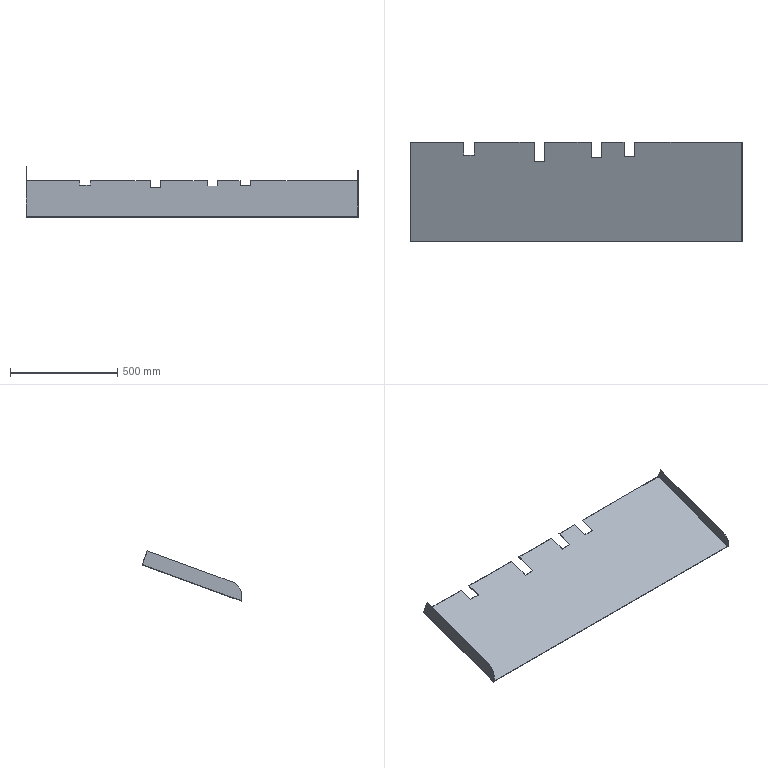Part | NX | features solid 2 | 1 solid | 28 faces | box 1550 x 466.287 x 233.957 mm | volume 1602943 mm3 | plane 26 | cylinder 2 | commonest cylinder face diameters 100 x1 140 x1
STEP:
#1=CARTESIAN_POINT('',(-650.,-738.618,-498.246));
#2=VERTEX_POINT('',#1);
#3=CARTESIAN_POINT('',(-370.,-738.618,-498.246));
#4=VERTEX_POINT('',#3);
#5=CARTESIAN_POINT('',(108.81,-738.618,-498.246));
#6=DIRECTION('',(-1.,0.,0.));
#7=VECTOR('',#6,1000.);
#8=LINE('',#5,#7);
#9=EDGE_CURVE('',#2,#4,#8,.F.);
#10=ORIENTED_EDGE('',*,*,#9,.T.);
#11=CARTESIAN_POINT('',(-370.,-737.934,-500.125));
#12=VERTEX_POINT('',#11);
#13=CARTESIAN_POINT('',(-370.,-738.618,-498.246));
#14=DIRECTION('',(0.,-0.342,0.9397));
#15=VECTOR('',#14,1000.);
#16=LINE('',#13,#15);
#17=EDGE_CURVE('',#4,#12,#16,.F.);
#18=ORIENTED_EDGE('',*,*,#17,.T.);
#19=CARTESIAN_POINT('',(-650.,-737.934,-500.125));
#20=VERTEX_POINT('',#19);
#21=CARTESIAN_POINT('',(108.81,-737.934,-500.125));
#22=DIRECTION('',(-1.,0.,0.));
#23=VECTOR('',#22,1000.);
#24=LINE('',#21,#23);
#25=EDGE_CURVE('',#20,#12,#24,.F.);
#26=ORIENTED_EDGE('',*,*,#25,.F.);
#27=CARTESIAN_POINT('',(-650.,-738.618,-498.246));
#28=DIRECTION('',(0.,-0.342,0.9397));
#29=VECTOR('',#28,1000.);
#30=LINE('',#27,#29);
#31=EDGE_CURVE('',#20,#2,#30,.T.);
#32=ORIENTED_EDGE('',*,*,#31,.T.);
#33=EDGE_LOOP('',(#10,#18,#26,#32));
#34=FACE_BOUND('',#33,.T.);
#35=CARTESIAN_POINT('',(108.81,-738.618,-498.246));
#36=DIRECTION('',(0.,0.9397,0.342));
#37=DIRECTION('',(1.,0.,0.));
#38=AXIS2_PLACEMENT_3D('',#35,#36,#37);
#39=PLANE('',#38);
#40=ADVANCED_FACE('',(#34),#39,.T.);
#41=CARTESIAN_POINT('',(-55.,-737.934,-500.125));
#42=VERTEX_POINT('',#41);
#43=CARTESIAN_POINT('',(49.,-737.934,-500.125));
#44=VERTEX_POINT('',#43);
#45=CARTESIAN_POINT('',(108.81,-737.934,-500.125));
#46=DIRECTION('',(-1.,0.,0.));
#47=VECTOR('',#46,1000.);
#48=LINE('',#45,#47);
#49=EDGE_CURVE('',#42,#44,#48,.F.);
#50=ORIENTED_EDGE('',*,*,#49,.F.);
#51=CARTESIAN_POINT('',(-55.,-738.618,-498.246));
#52=VERTEX_POINT('',#51);
#53=CARTESIAN_POINT('',(-55.,-738.618,-498.246));
#54=DIRECTION('',(0.,-0.342,0.9397));
#55=VECTOR('',#54,1000.);
#56=LINE('',#53,#55);
#57=EDGE_CURVE('',#42,#52,#56,.T.);
#58=ORIENTED_EDGE('',*,*,#57,.T.);
#59=CARTESIAN_POINT('',(49.,-738.618,-498.246));
#60=VERTEX_POINT('',#59);
#61=CARTESIAN_POINT('',(108.81,-738.618,-498.246));
#62=DIRECTION('',(-1.,0.,0.));
#63=VECTOR('',#62,1000.);
#64=LINE('',#61,#63);
#65=EDGE_CURVE('',#52,#60,#64,.F.);
#66=ORIENTED_EDGE('',*,*,#65,.T.);
#67=CARTESIAN_POINT('',(49.,-738.618,-498.246));
#68=DIRECTION('',(0.,0.342,-0.9397));
#69=VECTOR('',#68,1000.);
#70=LINE('',#67,#69);
#71=EDGE_CURVE('',#60,#44,#70,.T.);
#72=ORIENTED_EDGE('',*,*,#71,.T.);
#73=EDGE_LOOP('',(#50,#58,#66,#72));
#74=FACE_BOUND('',#73,.T.);
#75=CARTESIAN_POINT('',(108.81,-738.618,-498.246));
#76=DIRECTION('',(0.,0.9397,0.342));
#77=DIRECTION('',(1.,0.,0.));
#78=AXIS2_PLACEMENT_3D('',#75,#76,#77);
#79=PLANE('',#78);
#80=ADVANCED_FACE('',(#74),#79,.T.);
#81=CARTESIAN_POINT('',(-320.,-737.934,-500.125));
#82=VERTEX_POINT('',#81);
#83=CARTESIAN_POINT('',(-105.,-737.934,-500.125));
#84=VERTEX_POINT('',#83);
#85=CARTESIAN_POINT('',(108.81,-737.934,-500.125));
#86=DIRECTION('',(-1.,0.,0.));
#87=VECTOR('',#86,1000.);
#88=LINE('',#85,#87);
#89=EDGE_CURVE('',#82,#84,#88,.F.);
#90=ORIENTED_EDGE('',*,*,#89,.F.);
#91=CARTESIAN_POINT('',(-320.,-738.618,-498.246));
#92=VERTEX_POINT('',#91);
#93=CARTESIAN_POINT('',(-320.,-738.618,-498.246));
#94=DIRECTION('',(0.,-0.342,0.9397));
#95=VECTOR('',#94,1000.);
#96=LINE('',#93,#95);
#97=EDGE_CURVE('',#82,#92,#96,.T.);
#98=ORIENTED_EDGE('',*,*,#97,.T.);
#99=CARTESIAN_POINT('',(-105.,-738.618,-498.246));
#100=VERTEX_POINT('',#99);
#101=CARTESIAN_POINT('',(108.81,-738.618,-498.246));
#102=DIRECTION('',(-1.,0.,0.));
#103=VECTOR('',#102,1000.);
#104=LINE('',#101,#103);
#105=EDGE_CURVE('',#92,#100,#104,.F.);
#106=ORIENTED_EDGE('',*,*,#105,.T.);
#107=CARTESIAN_POINT('',(-105.,-738.618,-498.246));
#108=DIRECTION('',(0.,-0.342,0.9397));
#109=VECTOR('',#108,1000.);
#110=LINE('',#107,#109);
#111=EDGE_CURVE('',#100,#84,#110,.F.);
#112=ORIENTED_EDGE('',*,*,#111,.T.);
#113=EDGE_LOOP('',(#90,#98,#106,#112));
#114=FACE_BOUND('',#113,.T.);
#115=CARTESIAN_POINT('',(108.81,-738.618,-498.246));
#116=DIRECTION('',(0.,0.9397,0.342));
#117=DIRECTION('',(1.,0.,0.));
#118=AXIS2_PLACEMENT_3D('',#115,#116,#117);
#119=PLANE('',#118);
#120=ADVANCED_FACE('',(#114),#119,.T.);
#121=CARTESIAN_POINT('',(-948.,-738.618,-498.246));
#122=VERTEX_POINT('',#121);
#123=CARTESIAN_POINT('',(-700.,-738.618,-498.246));
#124=VERTEX_POINT('',#123);
#125=CARTESIAN_POINT('',(108.81,-738.618,-498.246));
#126=DIRECTION('',(-1.,0.,0.));
#127=VECTOR('',#126,1000.);
#128=LINE('',#125,#127);
#129=EDGE_CURVE('',#122,#124,#128,.F.);
#130=ORIENTED_EDGE('',*,*,#129,.T.);
#131=CARTESIAN_POINT('',(-700.,-737.934,-500.125));
#132=VERTEX_POINT('',#131);
#133=CARTESIAN_POINT('',(-700.,-738.618,-498.246));
#134=DIRECTION('',(0.,-0.342,0.9397));
#135=VECTOR('',#134,1000.);
#136=LINE('',#133,#135);
#137=EDGE_CURVE('',#124,#132,#136,.F.);
#138=ORIENTED_EDGE('',*,*,#137,.T.);
#139=CARTESIAN_POINT('',(-950.,-737.934,-500.125));
#140=VERTEX_POINT('',#139);
#141=CARTESIAN_POINT('',(108.81,-737.934,-500.125));
#142=DIRECTION('',(-1.,0.,0.));
#143=VECTOR('',#142,1000.);
#144=LINE('',#141,#143);
#145=EDGE_CURVE('',#140,#132,#144,.F.);
#146=ORIENTED_EDGE('',*,*,#145,.F.);
#147=CARTESIAN_POINT('',(-950.,-761.876,-434.347));
#148=VERTEX_POINT('',#147);
#149=CARTESIAN_POINT('',(-950.,-745.859,-478.352));
#150=DIRECTION('',(0.,-0.342,0.9397));
#151=VECTOR('',#150,1000.);
#152=LINE('',#149,#151);
#153=EDGE_CURVE('',#148,#140,#152,.F.);
#154=ORIENTED_EDGE('',*,*,#153,.F.);
#155=CARTESIAN_POINT('',(-948.,-761.876,-434.347));
#156=VERTEX_POINT('',#155);
#157=CARTESIAN_POINT('',(-950.,-761.876,-434.347));
#158=DIRECTION('',(1.,0.,0.));
#159=VECTOR('',#158,1000.);
#160=LINE('',#157,#159);
#161=EDGE_CURVE('',#148,#156,#160,.T.);
#162=ORIENTED_EDGE('',*,*,#161,.T.);
#163=CARTESIAN_POINT('',(-948.,-737.934,-500.125));
#164=DIRECTION('',(0.,0.342,-0.9397));
#165=VECTOR('',#164,1000.);
#166=LINE('',#163,#165);
#167=EDGE_CURVE('',#122,#156,#166,.F.);
#168=ORIENTED_EDGE('',*,*,#167,.F.);
#169=EDGE_LOOP('',(#130,#138,#146,#154,#162,#168));
#170=FACE_BOUND('',#169,.T.);
#171=CARTESIAN_POINT('',(108.81,-738.618,-498.246));
#172=DIRECTION('',(0.,0.9397,0.342));
#173=DIRECTION('',(1.,0.,0.));
#174=AXIS2_PLACEMENT_3D('',#171,#172,#173);
#175=PLANE('',#174);
#176=ADVANCED_FACE('',(#170),#175,.T.);
#177=CARTESIAN_POINT('',(-948.,-1200.,-668.304));
#178=VERTEX_POINT('',#177);
#179=CARTESIAN_POINT('',(597.803,-1200.,-668.304));
#180=VERTEX_POINT('',#179);
#181=CARTESIAN_POINT('',(108.81,-1200.,-668.304));
#182=DIRECTION('',(1.,0.,0.));
#183=VECTOR('',#182,1000.);
#184=LINE('',#181,#183);
#185=EDGE_CURVE('',#178,#180,#184,.T.);
#186=ORIENTED_EDGE('',*,*,#185,.T.);
#187=CARTESIAN_POINT('',(597.803,-1200.,-666.175));
#188=VERTEX_POINT('',#187);
#189=CARTESIAN_POINT('',(597.803,-1200.,-700.));
#190=DIRECTION('',(0.,0.,1.));
#191=VECTOR('',#190,1000.);
#192=LINE('',#189,#191);
#193=EDGE_CURVE('',#180,#188,#192,.T.);
#194=ORIENTED_EDGE('',*,*,#193,.T.);
#195=CARTESIAN_POINT('',(-948.,-1200.,-666.175));
#196=VERTEX_POINT('',#195);
#197=CARTESIAN_POINT('',(108.81,-1200.,-666.175));
#198=DIRECTION('',(1.,0.,0.));
#199=VECTOR('',#198,1000.);
#200=LINE('',#197,#199);
#201=EDGE_CURVE('',#196,#188,#200,.T.);
#202=ORIENTED_EDGE('',*,*,#201,.F.);
#203=CARTESIAN_POINT('',(-948.,-1200.,-700.));
#204=DIRECTION('',(0.,0.,1.));
#205=VECTOR('',#204,1000.);
#206=LINE('',#203,#205);
#207=EDGE_CURVE('',#178,#196,#206,.T.);
#208=ORIENTED_EDGE('',*,*,#207,.F.);
#209=EDGE_LOOP('',(#186,#194,#202,#208));
#210=FACE_BOUND('',#209,.T.);
#211=CARTESIAN_POINT('',(-1915.,-1200.,-700.));
#212=DIRECTION('',(0.,1.,0.));
#213=DIRECTION('',(-1.,0.,0.));
#214=AXIS2_PLACEMENT_3D('',#211,#212,#213);
#215=PLANE('',#214);
#216=ADVANCED_FACE('',(#210),#215,.F.);
#217=CARTESIAN_POINT('',(-370.,-830.,-531.506));
#218=VERTEX_POINT('',#217);
#219=CARTESIAN_POINT('',(-320.,-830.,-531.506));
#220=VERTEX_POINT('',#219);
#221=CARTESIAN_POINT('',(108.81,-830.,-531.506));
#222=DIRECTION('',(1.,0.,0.));
#223=VECTOR('',#222,1000.);
#224=LINE('',#221,#223);
#225=EDGE_CURVE('',#218,#220,#224,.T.);
#226=ORIENTED_EDGE('',*,*,#225,.F.);
#227=CARTESIAN_POINT('',(-370.,-818.492,-527.318));
#228=DIRECTION('',(0.,0.9397,0.342));
#229=VECTOR('',#228,1000.);
#230=LINE('',#227,#229);
#231=EDGE_CURVE('',#218,#4,#230,.T.);
#232=ORIENTED_EDGE('',*,*,#231,.T.);
#233=ORIENTED_EDGE('',*,*,#9,.F.);
#234=CARTESIAN_POINT('',(-650.,-798.905,-520.189));
#235=VERTEX_POINT('',#234);
#236=CARTESIAN_POINT('',(-650.,-818.492,-527.318));
#237=DIRECTION('',(0.,0.9397,0.342));
#238=VECTOR('',#237,1000.);
#239=LINE('',#236,#238);
#240=EDGE_CURVE('',#2,#235,#239,.F.);
#241=ORIENTED_EDGE('',*,*,#240,.T.);
#242=CARTESIAN_POINT('',(-700.,-798.905,-520.189));
#243=VERTEX_POINT('',#242);
#244=CARTESIAN_POINT('',(108.81,-798.905,-520.189));
#245=DIRECTION('',(1.,0.,0.));
#246=VECTOR('',#245,1000.);
#247=LINE('',#244,#246);
#248=EDGE_CURVE('',#235,#243,#247,.F.);
#249=ORIENTED_EDGE('',*,*,#248,.T.);
#250=CARTESIAN_POINT('',(-700.,-818.492,-527.318));
#251=DIRECTION('',(0.,0.9397,0.342));
#252=VECTOR('',#251,1000.);
#253=LINE('',#250,#252);
#254=EDGE_CURVE('',#243,#124,#253,.T.);
#255=ORIENTED_EDGE('',*,*,#254,.T.);
#256=ORIENTED_EDGE('',*,*,#129,.F.);
#257=CARTESIAN_POINT('',(-948.,-818.492,-527.318));
#258=DIRECTION('',(0.,0.9397,0.342));
#259=VECTOR('',#258,1000.);
#260=LINE('',#257,#259);
#261=EDGE_CURVE('',#196,#122,#260,.T.);
#262=ORIENTED_EDGE('',*,*,#261,.F.);
#263=ORIENTED_EDGE('',*,*,#201,.T.);
#264=CARTESIAN_POINT('',(597.803,-738.618,-498.246));
#265=VERTEX_POINT('',#264);
#266=CARTESIAN_POINT('',(597.803,-818.492,-527.318));
#267=DIRECTION('',(0.,0.9397,0.342));
#268=VECTOR('',#267,1000.);
#269=LINE('',#266,#268);
#270=EDGE_CURVE('',#188,#265,#269,.T.);
#271=ORIENTED_EDGE('',*,*,#270,.T.);
#272=CARTESIAN_POINT('',(99.,-738.618,-498.246));
#273=VERTEX_POINT('',#272);
#274=CARTESIAN_POINT('',(108.81,-738.618,-498.246));
#275=DIRECTION('',(-1.,0.,0.));
#276=VECTOR('',#275,1000.);
#277=LINE('',#274,#276);
#278=EDGE_CURVE('',#273,#265,#277,.F.);
#279=ORIENTED_EDGE('',*,*,#278,.F.);
#280=CARTESIAN_POINT('',(99.,-804.654,-522.281));
#281=VERTEX_POINT('',#280);
#282=CARTESIAN_POINT('',(99.,-818.492,-527.318));
#283=DIRECTION('',(0.,-0.9397,-0.342));
#284=VECTOR('',#283,1000.);
#285=LINE('',#282,#284);
#286=EDGE_CURVE('',#273,#281,#285,.T.);
#287=ORIENTED_EDGE('',*,*,#286,.T.);
#288=CARTESIAN_POINT('',(49.,-804.654,-522.281));
#289=VERTEX_POINT('',#288);
#290=CARTESIAN_POINT('',(108.81,-804.654,-522.281));
#291=DIRECTION('',(-1.,0.,0.));
#292=VECTOR('',#291,1000.);
#293=LINE('',#290,#292);
#294=EDGE_CURVE('',#281,#289,#293,.T.);
#295=ORIENTED_EDGE('',*,*,#294,.T.);
#296=CARTESIAN_POINT('',(49.,-818.492,-527.318));
#297=DIRECTION('',(0.,-0.9397,-0.342));
#298=VECTOR('',#297,1000.);
#299=LINE('',#296,#298);
#300=EDGE_CURVE('',#289,#60,#299,.F.);
#301=ORIENTED_EDGE('',*,*,#300,.T.);
#302=ORIENTED_EDGE('',*,*,#65,.F.);
#303=CARTESIAN_POINT('',(-55.,-809.9,-524.19));
#304=VERTEX_POINT('',#303);
#305=CARTESIAN_POINT('',(-55.,-818.492,-527.318));
#306=DIRECTION('',(0.,0.9397,0.342));
#307=VECTOR('',#306,1000.);
#308=LINE('',#305,#307);
#309=EDGE_CURVE('',#52,#304,#308,.F.);
#310=ORIENTED_EDGE('',*,*,#309,.T.);
#311=CARTESIAN_POINT('',(-105.,-809.9,-524.19));
#312=VERTEX_POINT('',#311);
#313=CARTESIAN_POINT('',(108.81,-809.9,-524.19));
#314=DIRECTION('',(-1.,0.,0.));
#315=VECTOR('',#314,1000.);
#316=LINE('',#313,#315);
#317=EDGE_CURVE('',#304,#312,#316,.T.);
#318=ORIENTED_EDGE('',*,*,#317,.T.);
#319=CARTESIAN_POINT('',(-105.,-818.492,-527.318));
#320=DIRECTION('',(0.,0.9397,0.342));
#321=VECTOR('',#320,1000.);
#322=LINE('',#319,#321);
#323=EDGE_CURVE('',#312,#100,#322,.T.);
#324=ORIENTED_EDGE('',*,*,#323,.T.);
#325=ORIENTED_EDGE('',*,*,#105,.F.);
#326=CARTESIAN_POINT('',(-320.,-818.492,-527.318));
#327=DIRECTION('',(0.,0.9397,0.342));
#328=VECTOR('',#327,1000.);
#329=LINE('',#326,#328);
#330=EDGE_CURVE('',#92,#220,#329,.F.);
#331=ORIENTED_EDGE('',*,*,#330,.T.);
#332=EDGE_LOOP('',(#226,#232,#233,#241,#249,#255,#256,#262,#263,#271,#279,#287,#295,#301,#302,#310,#318,#324,#325,#331));
#333=FACE_BOUND('',#332,.T.);
#334=CARTESIAN_POINT('',(108.81,-818.492,-527.318));
#335=DIRECTION('',(0.,0.342,-0.9397));
#336=DIRECTION('',(-1.,0.,0.));
#337=AXIS2_PLACEMENT_3D('',#334,#335,#336);
#338=PLANE('',#337);
#339=ADVANCED_FACE('',(#333),#338,.F.);
#340=CARTESIAN_POINT('',(99.,-737.934,-500.125));
#341=VERTEX_POINT('',#340);
#342=CARTESIAN_POINT('',(599.803,-737.934,-500.125));
#343=VERTEX_POINT('',#342);
#344=CARTESIAN_POINT('',(108.81,-737.934,-500.125));
#345=DIRECTION('',(-1.,0.,0.));
#346=VECTOR('',#345,1000.);
#347=LINE('',#344,#346);
#348=EDGE_CURVE('',#341,#343,#347,.F.);
#349=ORIENTED_EDGE('',*,*,#348,.F.);
#350=CARTESIAN_POINT('',(99.,-738.618,-498.246));
#351=DIRECTION('',(0.,0.342,-0.9397));
#352=VECTOR('',#351,1000.);
#353=LINE('',#350,#352);
#354=EDGE_CURVE('',#341,#273,#353,.F.);
#355=ORIENTED_EDGE('',*,*,#354,.T.);
#356=ORIENTED_EDGE('',*,*,#278,.T.);
#357=CARTESIAN_POINT('',(597.803,-755.035,-453.141));
#358=VERTEX_POINT('',#357);
#359=CARTESIAN_POINT('',(597.803,-737.934,-500.125));
#360=DIRECTION('',(0.,-0.342,0.9397));
#361=VECTOR('',#360,1000.);
#362=LINE('',#359,#361);
#363=EDGE_CURVE('',#265,#358,#362,.T.);
#364=ORIENTED_EDGE('',*,*,#363,.T.);
#365=CARTESIAN_POINT('',(599.803,-755.035,-453.141));
#366=VERTEX_POINT('',#365);
#367=CARTESIAN_POINT('',(599.803,-755.035,-453.141));
#368=DIRECTION('',(-1.,0.,0.));
#369=VECTOR('',#368,1000.);
#370=LINE('',#367,#369);
#371=EDGE_CURVE('',#366,#358,#370,.T.);
#372=ORIENTED_EDGE('',*,*,#371,.F.);
#373=CARTESIAN_POINT('',(599.803,-738.618,-498.246));
#374=DIRECTION('',(0.,0.342,-0.9397));
#375=VECTOR('',#374,1000.);
#376=LINE('',#373,#375);
#377=EDGE_CURVE('',#366,#343,#376,.T.);
#378=ORIENTED_EDGE('',*,*,#377,.T.);
#379=EDGE_LOOP('',(#349,#355,#356,#364,#372,#378));
#380=FACE_BOUND('',#379,.T.);
#381=CARTESIAN_POINT('',(108.81,-738.618,-498.246));
#382=DIRECTION('',(0.,0.9397,0.342));
#383=DIRECTION('',(1.,0.,0.));
#384=AXIS2_PLACEMENT_3D('',#381,#382,#383);
#385=PLANE('',#384);
#386=ADVANCED_FACE('',(#380),#385,.T.);
#387=CARTESIAN_POINT('',(-950.,-1200.,-668.304));
#388=VERTEX_POINT('',#387);
#389=CARTESIAN_POINT('',(-950.,-817.808,-529.197));
#390=DIRECTION('',(0.,-0.9397,-0.342));
#391=VECTOR('',#390,1000.);
#392=LINE('',#389,#391);
#393=EDGE_CURVE('',#140,#388,#392,.T.);
#394=ORIENTED_EDGE('',*,*,#393,.T.);
#395=CARTESIAN_POINT('',(-950.,-1158.163,-578.584));
#396=VERTEX_POINT('',#395);
#397=CARTESIAN_POINT('',(-950.,-1134.222,-644.362));
#398=DIRECTION('',(-1.,0.,0.));
#399=DIRECTION('',(0.,0.,1.));
#400=AXIS2_PLACEMENT_3D('',#397,#398,#399);
#401=CIRCLE('',#400,70.);
#402=EDGE_CURVE('',#388,#396,#401,.T.);
#403=ORIENTED_EDGE('',*,*,#402,.T.);
#404=CARTESIAN_POINT('',(-950.,-808.86,-451.448));
#405=DIRECTION('',(0.,0.9397,0.342));
#406=VECTOR('',#405,1000.);
#407=LINE('',#404,#406);
#408=EDGE_CURVE('',#148,#396,#407,.F.);
#409=ORIENTED_EDGE('',*,*,#408,.F.);
#410=ORIENTED_EDGE('',*,*,#153,.T.);
#411=EDGE_LOOP('',(#394,#403,#409,#410));
#412=FACE_BOUND('',#411,.T.);
#413=CARTESIAN_POINT('',(-950.,-1099.866,-607.2));
#414=DIRECTION('',(1.,0.,0.));
#415=DIRECTION('',(0.,0.,-1.));
#416=AXIS2_PLACEMENT_3D('',#413,#414,#415);
#417=PLANE('',#416);
#418=ADVANCED_FACE('',(#412),#417,.F.);
#419=CARTESIAN_POINT('',(599.803,-1170.116,-604.218));
#420=VERTEX_POINT('',#419);
#421=CARTESIAN_POINT('',(599.803,-1200.,-668.304));
#422=VERTEX_POINT('',#421);
#423=CARTESIAN_POINT('',(599.803,-1153.015,-651.203));
#424=DIRECTION('',(-1.,0.,0.));
#425=DIRECTION('',(0.,0.,1.));
#426=AXIS2_PLACEMENT_3D('',#423,#424,#425);
#427=CIRCLE('',#426,50.);
#428=EDGE_CURVE('',#420,#422,#427,.F.);
#429=ORIENTED_EDGE('',*,*,#428,.T.);
#430=CARTESIAN_POINT('',(599.803,-817.808,-529.197));
#431=DIRECTION('',(0.,0.9397,0.342));
#432=VECTOR('',#431,1000.);
#433=LINE('',#430,#432);
#434=EDGE_CURVE('',#343,#422,#433,.F.);
#435=ORIENTED_EDGE('',*,*,#434,.F.);
#436=ORIENTED_EDGE('',*,*,#377,.F.);
#437=CARTESIAN_POINT('',(599.803,-811.417,-473.662));
#438=DIRECTION('',(0.,-0.9397,-0.342));
#439=VECTOR('',#438,1000.);
#440=LINE('',#437,#439);
#441=EDGE_CURVE('',#366,#420,#440,.T.);
#442=ORIENTED_EDGE('',*,*,#441,.T.);
#443=EDGE_LOOP('',(#429,#435,#436,#442));
#444=FACE_BOUND('',#443,.T.);
#445=CARTESIAN_POINT('',(599.803,-818.492,-527.318));
#446=DIRECTION('',(1.,0.,0.));
#447=DIRECTION('',(0.,-0.9397,-0.342));
#448=AXIS2_PLACEMENT_3D('',#445,#446,#447);
#449=PLANE('',#448);
#450=ADVANCED_FACE('',(#444),#449,.T.);
#451=CARTESIAN_POINT('',(-370.,-830.,-533.635));
#452=VERTEX_POINT('',#451);
#453=CARTESIAN_POINT('',(-370.,-817.808,-529.197));
#454=DIRECTION('',(0.,0.9397,0.342));
#455=VECTOR('',#454,1000.);
#456=LINE('',#453,#455);
#457=EDGE_CURVE('',#452,#12,#456,.T.);
#458=ORIENTED_EDGE('',*,*,#457,.F.);
#459=CARTESIAN_POINT('',(-320.,-830.,-533.635));
#460=VERTEX_POINT('',#459);
#461=CARTESIAN_POINT('',(108.81,-830.,-533.635));
#462=DIRECTION('',(1.,0.,0.));
#463=VECTOR('',#462,1000.);
#464=LINE('',#461,#463);
#465=EDGE_CURVE('',#452,#460,#464,.T.);
#466=ORIENTED_EDGE('',*,*,#465,.T.);
#467=CARTESIAN_POINT('',(-320.,-817.808,-529.197));
#468=DIRECTION('',(0.,0.9397,0.342));
#469=VECTOR('',#468,1000.);
#470=LINE('',#467,#469);
#471=EDGE_CURVE('',#82,#460,#470,.F.);
#472=ORIENTED_EDGE('',*,*,#471,.F.);
#473=ORIENTED_EDGE('',*,*,#89,.T.);
#474=CARTESIAN_POINT('',(-105.,-810.264,-526.451));
#475=VERTEX_POINT('',#474);
#476=CARTESIAN_POINT('',(-105.,-817.808,-529.197));
#477=DIRECTION('',(0.,0.9397,0.342));
#478=VECTOR('',#477,1000.);
#479=LINE('',#476,#478);
#480=EDGE_CURVE('',#475,#84,#479,.T.);
#481=ORIENTED_EDGE('',*,*,#480,.F.);
#482=CARTESIAN_POINT('',(-55.,-810.264,-526.451));
#483=VERTEX_POINT('',#482);
#484=CARTESIAN_POINT('',(108.81,-810.264,-526.451));
#485=DIRECTION('',(-1.,0.,0.));
#486=VECTOR('',#485,1000.);
#487=LINE('',#484,#486);
#488=EDGE_CURVE('',#483,#475,#487,.T.);
#489=ORIENTED_EDGE('',*,*,#488,.F.);
#490=CARTESIAN_POINT('',(-55.,-817.808,-529.197));
#491=DIRECTION('',(0.,0.9397,0.342));
#492=VECTOR('',#491,1000.);
#493=LINE('',#490,#492);
#494=EDGE_CURVE('',#42,#483,#493,.F.);
#495=ORIENTED_EDGE('',*,*,#494,.F.);
#496=ORIENTED_EDGE('',*,*,#49,.T.);
#497=CARTESIAN_POINT('',(49.,-805.113,-524.577));
#498=VERTEX_POINT('',#497);
#499=CARTESIAN_POINT('',(49.,-817.808,-529.197));
#500=DIRECTION('',(0.,-0.9397,-0.342));
#501=VECTOR('',#500,1000.);
#502=LINE('',#499,#501);
#503=EDGE_CURVE('',#498,#44,#502,.F.);
#504=ORIENTED_EDGE('',*,*,#503,.F.);
#505=CARTESIAN_POINT('',(99.,-805.113,-524.577));
#506=VERTEX_POINT('',#505);
#507=CARTESIAN_POINT('',(108.81,-805.113,-524.577));
#508=DIRECTION('',(-1.,0.,0.));
#509=VECTOR('',#508,1000.);
#510=LINE('',#507,#509);
#511=EDGE_CURVE('',#506,#498,#510,.T.);
#512=ORIENTED_EDGE('',*,*,#511,.F.);
#513=CARTESIAN_POINT('',(99.,-817.808,-529.197));
#514=DIRECTION('',(0.,-0.9397,-0.342));
#515=VECTOR('',#514,1000.);
#516=LINE('',#513,#515);
#517=EDGE_CURVE('',#341,#506,#516,.T.);
#518=ORIENTED_EDGE('',*,*,#517,.F.);
#519=ORIENTED_EDGE('',*,*,#348,.T.);
#520=ORIENTED_EDGE('',*,*,#434,.T.);
#521=CARTESIAN_POINT('',(599.803,-1200.,-668.304));
#522=DIRECTION('',(1.,0.,0.));
#523=VECTOR('',#522,1000.);
#524=LINE('',#521,#523);
#525=EDGE_CURVE('',#422,#180,#524,.F.);
#526=ORIENTED_EDGE('',*,*,#525,.T.);
#527=ORIENTED_EDGE('',*,*,#185,.F.);
#528=CARTESIAN_POINT('',(108.81,-1200.,-668.304));
#529=DIRECTION('',(1.,0.,0.));
#530=VECTOR('',#529,1000.);
#531=LINE('',#528,#530);
#532=EDGE_CURVE('',#388,#178,#531,.T.);
#533=ORIENTED_EDGE('',*,*,#532,.F.);
#534=ORIENTED_EDGE('',*,*,#393,.F.);
#535=ORIENTED_EDGE('',*,*,#145,.T.);
#536=CARTESIAN_POINT('',(-700.,-799.469,-522.522));
#537=VERTEX_POINT('',#536);
#538=CARTESIAN_POINT('',(-700.,-817.808,-529.197));
#539=DIRECTION('',(0.,0.9397,0.342));
#540=VECTOR('',#539,1000.);
#541=LINE('',#538,#540);
#542=EDGE_CURVE('',#537,#132,#541,.T.);
#543=ORIENTED_EDGE('',*,*,#542,.F.);
#544=CARTESIAN_POINT('',(-650.,-799.469,-522.522));
#545=VERTEX_POINT('',#544);
#546=CARTESIAN_POINT('',(108.81,-799.469,-522.522));
#547=DIRECTION('',(1.,0.,0.));
#548=VECTOR('',#547,1000.);
#549=LINE('',#546,#548);
#550=EDGE_CURVE('',#545,#537,#549,.F.);
#551=ORIENTED_EDGE('',*,*,#550,.F.);
#552=CARTESIAN_POINT('',(-650.,-817.808,-529.197));
#553=DIRECTION('',(0.,0.9397,0.342));
#554=VECTOR('',#553,1000.);
#555=LINE('',#552,#554);
#556=EDGE_CURVE('',#20,#545,#555,.F.);
#557=ORIENTED_EDGE('',*,*,#556,.F.);
#558=ORIENTED_EDGE('',*,*,#25,.T.);
#559=EDGE_LOOP('',(#458,#466,#472,#473,#481,#489,#495,#496,#504,#512,#518,#519,#520,#526,#527,#533,#534,#535,#543,#551,#557,#558));
#560=FACE_BOUND('',#559,.T.);
#561=CARTESIAN_POINT('',(108.81,-817.808,-529.197));
#562=DIRECTION('',(0.,0.342,-0.9397));
#563=DIRECTION('',(-1.,0.,0.));
#564=AXIS2_PLACEMENT_3D('',#561,#562,#563);
#565=PLANE('',#564);
#566=ADVANCED_FACE('',(#560),#565,.T.);
#567=CARTESIAN_POINT('',(-948.,-1158.163,-578.584));
#568=VERTEX_POINT('',#567);
#569=CARTESIAN_POINT('',(-948.,-1134.222,-644.362));
#570=DIRECTION('',(-1.,0.,0.));
#571=DIRECTION('',(0.,0.,1.));
#572=AXIS2_PLACEMENT_3D('',#569,#570,#571);
#573=CIRCLE('',#572,70.);
#574=EDGE_CURVE('',#568,#178,#573,.F.);
#575=ORIENTED_EDGE('',*,*,#574,.T.);
#576=ORIENTED_EDGE('',*,*,#207,.T.);
#577=ORIENTED_EDGE('',*,*,#261,.T.);
#578=ORIENTED_EDGE('',*,*,#167,.T.);
#579=CARTESIAN_POINT('',(-948.,-808.86,-451.448));
#580=DIRECTION('',(0.,0.9397,0.342));
#581=VECTOR('',#580,1000.);
#582=LINE('',#579,#581);
#583=EDGE_CURVE('',#156,#568,#582,.F.);
#584=ORIENTED_EDGE('',*,*,#583,.T.);
#585=EDGE_LOOP('',(#575,#576,#577,#578,#584));
#586=FACE_BOUND('',#585,.T.);
#587=CARTESIAN_POINT('',(-948.,-784.919,-517.226));
#588=DIRECTION('',(-1.,0.,0.));
#589=DIRECTION('',(0.,0.,1.));
#590=AXIS2_PLACEMENT_3D('',#587,#588,#589);
#591=PLANE('',#590);
#592=ADVANCED_FACE('',(#586),#591,.F.);
#593=ORIENTED_EDGE('',*,*,#408,.T.);
#594=CARTESIAN_POINT('',(-950.,-1158.163,-578.584));
#595=DIRECTION('',(1.,0.,0.));
#596=VECTOR('',#595,1000.);
#597=LINE('',#594,#596);
#598=EDGE_CURVE('',#396,#568,#597,.T.);
#599=ORIENTED_EDGE('',*,*,#598,.T.);
#600=ORIENTED_EDGE('',*,*,#583,.F.);
#601=ORIENTED_EDGE('',*,*,#161,.F.);
#602=EDGE_LOOP('',(#593,#599,#600,#601));
#603=FACE_BOUND('',#602,.T.);
#604=CARTESIAN_POINT('',(-950.,-808.86,-451.448));
#605=DIRECTION('',(0.,0.342,-0.9397));
#606=DIRECTION('',(0.,-0.9397,-0.342));
#607=AXIS2_PLACEMENT_3D('',#604,#605,#606);
#608=PLANE('',#607);
#609=ADVANCED_FACE('',(#603),#608,.F.);
#610=ORIENTED_EDGE('',*,*,#402,.F.);
#611=ORIENTED_EDGE('',*,*,#532,.T.);
#612=ORIENTED_EDGE('',*,*,#574,.F.);
#613=ORIENTED_EDGE('',*,*,#598,.F.);
#614=EDGE_LOOP('',(#610,#611,#612,#613));
#615=FACE_BOUND('',#614,.T.);
#616=CARTESIAN_POINT('',(-950.,-1134.222,-644.362));
#617=DIRECTION('',(-1.,0.,0.));
#618=DIRECTION('',(0.,0.,1.));
#619=AXIS2_PLACEMENT_3D('',#616,#617,#618);
#620=CYLINDRICAL_SURFACE('',#619,70.);
#621=ADVANCED_FACE('',(#615),#620,.T.);
#622=ORIENTED_EDGE('',*,*,#193,.F.);
#623=CARTESIAN_POINT('',(597.803,-1170.116,-604.218));
#624=VERTEX_POINT('',#623);
#625=CARTESIAN_POINT('',(597.803,-1153.015,-651.203));
#626=DIRECTION('',(-1.,0.,0.));
#627=DIRECTION('',(0.,0.,1.));
#628=AXIS2_PLACEMENT_3D('',#625,#626,#627);
#629=CIRCLE('',#628,50.);
#630=EDGE_CURVE('',#180,#624,#629,.T.);
#631=ORIENTED_EDGE('',*,*,#630,.T.);
#632=CARTESIAN_POINT('',(597.803,-811.417,-473.662));
#633=DIRECTION('',(0.,-0.9397,-0.342));
#634=VECTOR('',#633,1000.);
#635=LINE('',#632,#634);
#636=EDGE_CURVE('',#358,#624,#635,.T.);
#637=ORIENTED_EDGE('',*,*,#636,.F.);
#638=ORIENTED_EDGE('',*,*,#363,.F.);
#639=ORIENTED_EDGE('',*,*,#270,.F.);
#640=EDGE_LOOP('',(#622,#631,#637,#638,#639));
#641=FACE_BOUND('',#640,.T.);
#642=CARTESIAN_POINT('',(597.803,-794.316,-520.647));
#643=DIRECTION('',(-1.,0.,0.));
#644=DIRECTION('',(0.,0.,1.));
#645=AXIS2_PLACEMENT_3D('',#642,#643,#644);
#646=PLANE('',#645);
#647=ADVANCED_FACE('',(#641),#646,.T.);
#648=ORIENTED_EDGE('',*,*,#636,.T.);
#649=CARTESIAN_POINT('',(599.803,-1170.116,-604.218));
#650=DIRECTION('',(1.,0.,0.));
#651=VECTOR('',#650,1000.);
#652=LINE('',#649,#651);
#653=EDGE_CURVE('',#624,#420,#652,.T.);
#654=ORIENTED_EDGE('',*,*,#653,.T.);
#655=ORIENTED_EDGE('',*,*,#441,.F.);
#656=ORIENTED_EDGE('',*,*,#371,.T.);
#657=EDGE_LOOP('',(#648,#654,#655,#656));
#658=FACE_BOUND('',#657,.T.);
#659=CARTESIAN_POINT('',(599.803,-811.417,-473.662));
#660=DIRECTION('',(0.,0.342,-0.9397));
#661=DIRECTION('',(0.,-0.9397,-0.342));
#662=AXIS2_PLACEMENT_3D('',#659,#660,#661);
#663=PLANE('',#662);
#664=ADVANCED_FACE('',(#658),#663,.F.);
#665=ORIENTED_EDGE('',*,*,#428,.F.);
#666=ORIENTED_EDGE('',*,*,#653,.F.);
#667=ORIENTED_EDGE('',*,*,#630,.F.);
#668=ORIENTED_EDGE('',*,*,#525,.F.);
#669=EDGE_LOOP('',(#665,#666,#667,#668));
#670=FACE_BOUND('',#669,.T.);
#671=CARTESIAN_POINT('',(599.803,-1153.015,-651.203));
#672=DIRECTION('',(1.,0.,0.));
#673=DIRECTION('',(0.,0.,-1.));
#674=AXIS2_PLACEMENT_3D('',#671,#672,#673);
#675=CYLINDRICAL_SURFACE('',#674,50.);
#676=ADVANCED_FACE('',(#670),#675,.T.);
#677=CARTESIAN_POINT('',(-650.,-698.573,-105.18));
#678=DIRECTION('',(0.,-0.235,-0.972));
#679=VECTOR('',#678,1000.);
#680=LINE('',#677,#679);
#681=EDGE_CURVE('',#235,#545,#680,.T.);
#682=ORIENTED_EDGE('',*,*,#681,.T.);
#683=ORIENTED_EDGE('',*,*,#550,.T.);
#684=CARTESIAN_POINT('',(-700.,-698.573,-105.18));
#685=DIRECTION('',(0.,-0.235,-0.972));
#686=VECTOR('',#685,1000.);
#687=LINE('',#684,#686);
#688=EDGE_CURVE('',#537,#243,#687,.F.);
#689=ORIENTED_EDGE('',*,*,#688,.T.);
#690=ORIENTED_EDGE('',*,*,#248,.F.);
#691=EDGE_LOOP('',(#682,#683,#689,#690));
#692=FACE_BOUND('',#691,.T.);
#693=CARTESIAN_POINT('',(-690.,-719.72,-192.65));
#694=DIRECTION('',(0.,0.972,-0.235));
#695=DIRECTION('',(0.,0.235,0.972));
#696=AXIS2_PLACEMENT_3D('',#693,#694,#695);
#697=PLANE('',#696);
#698=ADVANCED_FACE('',(#692),#697,.T.);
#699=ORIENTED_EDGE('',*,*,#31,.F.);
#700=ORIENTED_EDGE('',*,*,#556,.T.);
#701=ORIENTED_EDGE('',*,*,#681,.F.);
#702=ORIENTED_EDGE('',*,*,#240,.F.);
#703=EDGE_LOOP('',(#699,#700,#701,#702));
#704=FACE_BOUND('',#703,.T.);
#705=CARTESIAN_POINT('',(-650.,-720.,-100.));
#706=DIRECTION('',(-1.,0.,0.));
#707=DIRECTION('',(0.,0.,-1.));
#708=AXIS2_PLACEMENT_3D('',#705,#706,#707);
#709=PLANE('',#708);
#710=ADVANCED_FACE('',(#704),#709,.T.);
#711=ORIENTED_EDGE('',*,*,#688,.F.);
#712=ORIENTED_EDGE('',*,*,#542,.T.);
#713=ORIENTED_EDGE('',*,*,#137,.F.);
#714=ORIENTED_EDGE('',*,*,#254,.F.);
#715=EDGE_LOOP('',(#711,#712,#713,#714));
#716=FACE_BOUND('',#715,.T.);
#717=CARTESIAN_POINT('',(-700.,-720.,-100.));
#718=DIRECTION('',(-1.,0.,0.));
#719=DIRECTION('',(0.,0.,-1.));
#720=AXIS2_PLACEMENT_3D('',#717,#718,#719);
#721=PLANE('',#720);
#722=ADVANCED_FACE('',(#716),#721,.F.);
#723=ORIENTED_EDGE('',*,*,#354,.F.);
#724=ORIENTED_EDGE('',*,*,#517,.T.);
#725=CARTESIAN_POINT('',(99.,-720.19,-99.962));
#726=DIRECTION('',(0.,-0.1961,-0.9806));
#727=VECTOR('',#726,1000.);
#728=LINE('',#725,#727);
#729=EDGE_CURVE('',#281,#506,#728,.T.);
#730=ORIENTED_EDGE('',*,*,#729,.F.);
#731=ORIENTED_EDGE('',*,*,#286,.F.);
#732=EDGE_LOOP('',(#723,#724,#730,#731));
#733=FACE_BOUND('',#732,.T.);
#734=CARTESIAN_POINT('',(99.,-720.,-100.));
#735=DIRECTION('',(1.,0.,0.));
#736=DIRECTION('',(0.,0.,-1.));
#737=AXIS2_PLACEMENT_3D('',#734,#735,#736);
#738=PLANE('',#737);
#739=ADVANCED_FACE('',(#733),#738,.F.);
#740=ORIENTED_EDGE('',*,*,#729,.T.);
#741=ORIENTED_EDGE('',*,*,#511,.T.);
#742=CARTESIAN_POINT('',(49.,-720.19,-99.962));
#743=DIRECTION('',(0.,-0.1961,-0.9806));
#744=VECTOR('',#743,1000.);
#745=LINE('',#742,#744);
#746=EDGE_CURVE('',#498,#289,#745,.F.);
#747=ORIENTED_EDGE('',*,*,#746,.T.);
#748=ORIENTED_EDGE('',*,*,#294,.F.);
#749=EDGE_LOOP('',(#740,#741,#747,#748));
#750=FACE_BOUND('',#749,.T.);
#751=CARTESIAN_POINT('',(-1666.,-829.806,-648.039));
#752=DIRECTION('',(0.,-0.9806,0.1961));
#753=DIRECTION('',(0.,-0.1961,-0.9806));
#754=AXIS2_PLACEMENT_3D('',#751,#752,#753);
#755=PLANE('',#754);
#756=ADVANCED_FACE('',(#750),#755,.F.);
#757=ORIENTED_EDGE('',*,*,#746,.F.);
#758=ORIENTED_EDGE('',*,*,#503,.T.);
#759=ORIENTED_EDGE('',*,*,#71,.F.);
#760=ORIENTED_EDGE('',*,*,#300,.F.);
#761=EDGE_LOOP('',(#757,#758,#759,#760));
#762=FACE_BOUND('',#761,.T.);
#763=CARTESIAN_POINT('',(49.,-720.,-100.));
#764=DIRECTION('',(1.,0.,0.));
#765=DIRECTION('',(0.,0.,-1.));
#766=AXIS2_PLACEMENT_3D('',#763,#764,#765);
#767=PLANE('',#766);
#768=ADVANCED_FACE('',(#762),#767,.T.);
#769=CARTESIAN_POINT('',(-105.,-782.151,-351.604));
#770=DIRECTION('',(0.,0.1587,0.9873));
#771=VECTOR('',#770,1000.);
#772=LINE('',#769,#771);
#773=EDGE_CURVE('',#475,#312,#772,.T.);
#774=ORIENTED_EDGE('',*,*,#773,.F.);
#775=ORIENTED_EDGE('',*,*,#480,.T.);
#776=ORIENTED_EDGE('',*,*,#111,.F.);
#777=ORIENTED_EDGE('',*,*,#323,.F.);
#778=EDGE_LOOP('',(#774,#775,#776,#777));
#779=FACE_BOUND('',#778,.T.);
#780=CARTESIAN_POINT('',(-105.,-710.,-363.205));
#781=DIRECTION('',(-1.,0.,0.));
#782=DIRECTION('',(0.,0.,-1.));
#783=AXIS2_PLACEMENT_3D('',#780,#781,#782);
#784=PLANE('',#783);
#785=ADVANCED_FACE('',(#779),#784,.F.);
#786=CARTESIAN_POINT('',(-55.,-782.151,-351.604));
#787=DIRECTION('',(0.,0.1587,0.9873));
#788=VECTOR('',#787,1000.);
#789=LINE('',#786,#788);
#790=EDGE_CURVE('',#304,#483,#789,.F.);
#791=ORIENTED_EDGE('',*,*,#790,.T.);
#792=ORIENTED_EDGE('',*,*,#488,.T.);
#793=ORIENTED_EDGE('',*,*,#773,.T.);
#794=ORIENTED_EDGE('',*,*,#317,.F.);
#795=EDGE_LOOP('',(#791,#792,#793,#794));
#796=FACE_BOUND('',#795,.T.);
#797=CARTESIAN_POINT('',(1065.,-747.873,-138.413));
#798=DIRECTION('',(0.,-0.9873,0.1587));
#799=DIRECTION('',(0.,-0.1587,-0.9873));
#800=AXIS2_PLACEMENT_3D('',#797,#798,#799);
#801=PLANE('',#800);
#802=ADVANCED_FACE('',(#796),#801,.F.);
#803=ORIENTED_EDGE('',*,*,#57,.F.);
#804=ORIENTED_EDGE('',*,*,#494,.T.);
#805=ORIENTED_EDGE('',*,*,#790,.F.);
#806=ORIENTED_EDGE('',*,*,#309,.F.);
#807=EDGE_LOOP('',(#803,#804,#805,#806));
#808=FACE_BOUND('',#807,.T.);
#809=CARTESIAN_POINT('',(-55.,-710.,-363.205));
#810=DIRECTION('',(-1.,0.,0.));
#811=DIRECTION('',(0.,0.,-1.));
#812=AXIS2_PLACEMENT_3D('',#809,#810,#811);
#813=PLANE('',#812);
#814=ADVANCED_FACE('',(#808),#813,.T.);
#815=ORIENTED_EDGE('',*,*,#225,.T.);
#816=CARTESIAN_POINT('',(-320.,-830.,-700.));
#817=DIRECTION('',(0.,0.,1.));
#818=VECTOR('',#817,1000.);
#819=LINE('',#816,#818);
#820=EDGE_CURVE('',#220,#460,#819,.F.);
#821=ORIENTED_EDGE('',*,*,#820,.T.);
#822=ORIENTED_EDGE('',*,*,#465,.F.);
#823=CARTESIAN_POINT('',(-370.,-830.,-700.));
#824=DIRECTION('',(0.,0.,1.));
#825=VECTOR('',#824,1000.);
#826=LINE('',#823,#825);
#827=EDGE_CURVE('',#452,#218,#826,.T.);
#828=ORIENTED_EDGE('',*,*,#827,.T.);
#829=EDGE_LOOP('',(#815,#821,#822,#828));
#830=FACE_BOUND('',#829,.T.);
#831=CARTESIAN_POINT('',(1065.,-830.,-700.));
#832=DIRECTION('',(0.,1.,0.));
#833=DIRECTION('',(-1.,0.,0.));
#834=AXIS2_PLACEMENT_3D('',#831,#832,#833);
#835=PLANE('',#834);
#836=ADVANCED_FACE('',(#830),#835,.T.);
#837=ORIENTED_EDGE('',*,*,#827,.F.);
#838=ORIENTED_EDGE('',*,*,#457,.T.);
#839=ORIENTED_EDGE('',*,*,#17,.F.);
#840=ORIENTED_EDGE('',*,*,#231,.F.);
#841=EDGE_LOOP('',(#837,#838,#839,#840));
#842=FACE_BOUND('',#841,.T.);
#843=CARTESIAN_POINT('',(-370.,-710.,-363.208));
#844=DIRECTION('',(-1.,0.,0.));
#845=DIRECTION('',(0.,0.,-1.));
#846=AXIS2_PLACEMENT_3D('',#843,#844,#845);
#847=PLANE('',#846);
#848=ADVANCED_FACE('',(#842),#847,.F.);
#849=ORIENTED_EDGE('',*,*,#97,.F.);
#850=ORIENTED_EDGE('',*,*,#471,.T.);
#851=ORIENTED_EDGE('',*,*,#820,.F.);
#852=ORIENTED_EDGE('',*,*,#330,.F.);
#853=EDGE_LOOP('',(#849,#850,#851,#852));
#854=FACE_BOUND('',#853,.T.);
#855=CARTESIAN_POINT('',(-320.,-710.,-363.208));
#856=DIRECTION('',(-1.,0.,0.));
#857=DIRECTION('',(0.,0.,-1.));
#858=AXIS2_PLACEMENT_3D('',#855,#856,#857);
#859=PLANE('',#858);
#860=ADVANCED_FACE('',(#854),#859,.T.);
#861=CLOSED_SHELL('',(#40,#80,#120,#176,#216,#339,#386,#418,#450,#566,#592,#609,#621,#647,#664,#676,#698,#710,#722,#739,#756,#768,#785,#802,#814,#836,#848,#860));
#862=MANIFOLD_SOLID_BREP('',#861);
#863=(LENGTH_UNIT()NAMED_UNIT(*)SI_UNIT(.MILLI.,.METRE.));
#864=UNCERTAINTY_MEASURE_WITH_UNIT(LENGTH_MEASURE(0.00001),#863,'','');
#865=(NAMED_UNIT(*)PLANE_ANGLE_UNIT()SI_UNIT($,.RADIAN.));
#866=(NAMED_UNIT(*)SI_UNIT($,.STERADIAN.)SOLID_ANGLE_UNIT());
#867=(GEOMETRIC_REPRESENTATION_CONTEXT(3)GLOBAL_UNCERTAINTY_ASSIGNED_CONTEXT((#864))GLOBAL_UNIT_ASSIGNED_CONTEXT((#863,#865,#866))REPRESENTATION_CONTEXT('',''));
#868=ADVANCED_BREP_SHAPE_REPRESENTATION('',(#862),#867);